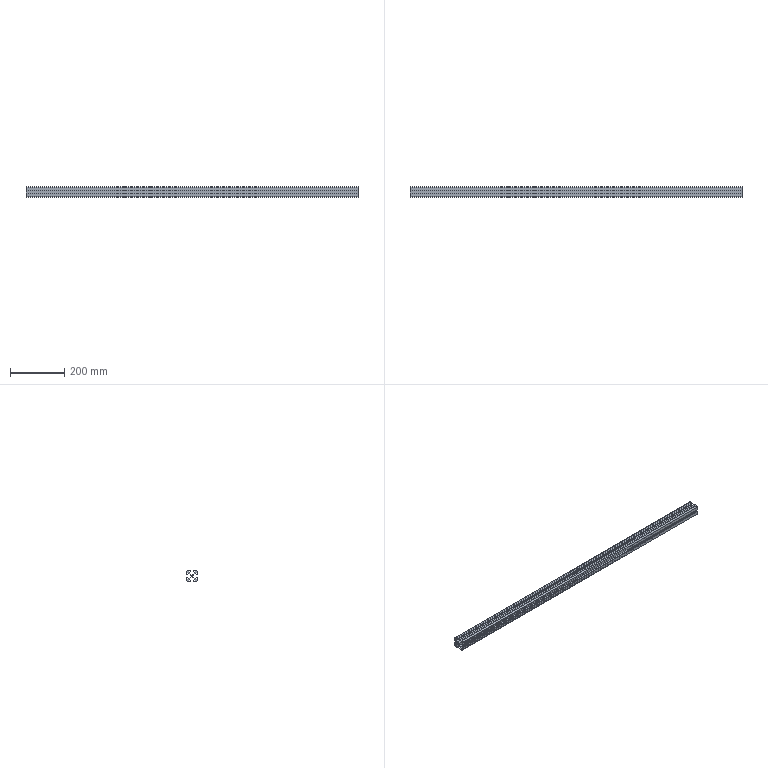Part | STEP file | 40x40-1220 | 1 solid | 67 faces | box 1220 x 40 x 40 mm | volume 673913 mm3 | plane 62 | cylinder 5 | commonest cylinder face diameters 9 x4 6.8 x1